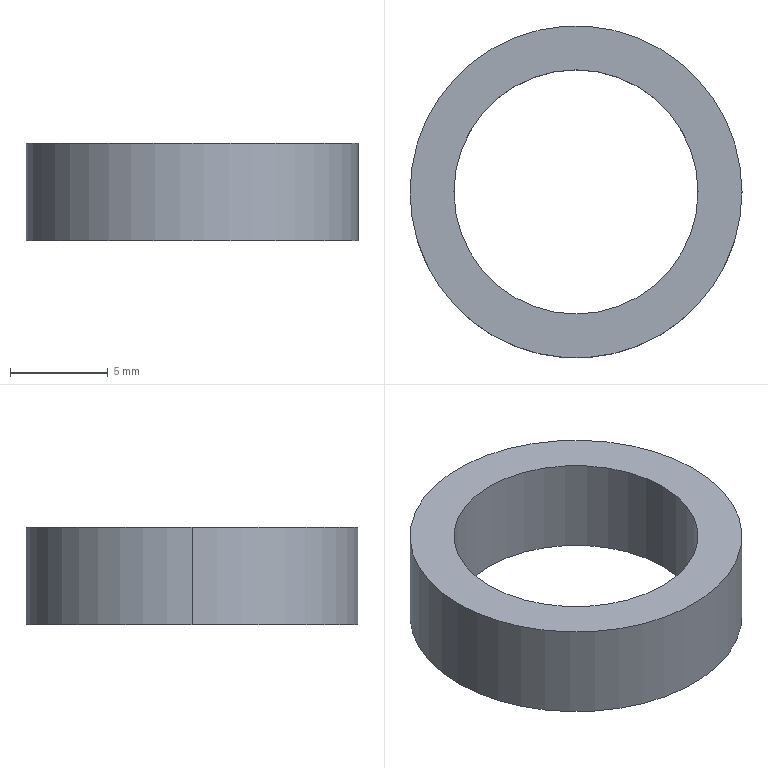Part | SolidWorks | features Extrusion 1 | 1 solid | 6 faces | box 17 x 17 x 5 mm | volume 521.308 mm3 | cylinder 4 | plane 2 | commonest cylinder face diameters 12.5 x2 17 x2
STEP:
#1=CARTESIAN_POINT('',(-6.25,0.,5.));
#2=VERTEX_POINT('',#1);
#3=CARTESIAN_POINT('',(6.25,0.,5.));
#4=VERTEX_POINT('',#3);
#5=CARTESIAN_POINT('',(0.,0.,5.));
#6=DIRECTION('',(0.,0.,1.));
#7=DIRECTION('',(1.,0.,0.));
#8=AXIS2_PLACEMENT_3D('',#5,#6,#7);
#9=CIRCLE('',#8,6.25);
#10=EDGE_CURVE('',#2,#4,#9,.T.);
#11=ORIENTED_EDGE('',*,*,#10,.T.);
#12=CARTESIAN_POINT('',(6.25,0.,0.));
#13=VERTEX_POINT('',#12);
#14=CARTESIAN_POINT('',(6.25,0.,5.));
#15=DIRECTION('',(0.,0.,-1.));
#16=VECTOR('',#15,1000.);
#17=LINE('',#14,#16);
#18=EDGE_CURVE('',#4,#13,#17,.T.);
#19=ORIENTED_EDGE('',*,*,#18,.T.);
#20=CARTESIAN_POINT('',(-6.25,0.,0.));
#21=VERTEX_POINT('',#20);
#22=CARTESIAN_POINT('',(0.,0.,0.));
#23=DIRECTION('',(0.,0.,1.));
#24=DIRECTION('',(1.,0.,0.));
#25=AXIS2_PLACEMENT_3D('',#22,#23,#24);
#26=CIRCLE('',#25,6.25);
#27=EDGE_CURVE('',#21,#13,#26,.T.);
#28=ORIENTED_EDGE('',*,*,#27,.F.);
#29=CARTESIAN_POINT('',(-6.25,0.,5.));
#30=DIRECTION('',(0.,0.,-1.));
#31=VECTOR('',#30,1000.);
#32=LINE('',#29,#31);
#33=EDGE_CURVE('',#2,#21,#32,.T.);
#34=ORIENTED_EDGE('',*,*,#33,.F.);
#35=EDGE_LOOP('',(#11,#19,#28,#34));
#36=FACE_OUTER_BOUND('',#35,.T.);
#37=CARTESIAN_POINT('',(0.,0.,5.));
#38=DIRECTION('',(0.,0.,-1.));
#39=DIRECTION('',(-1.,0.,0.));
#40=AXIS2_PLACEMENT_3D('',#37,#38,#39);
#41=CYLINDRICAL_SURFACE('',#40,6.25);
#42=ADVANCED_FACE('',(#36),#41,.F.);
#43=CARTESIAN_POINT('',(8.5,0.,5.));
#44=VERTEX_POINT('',#43);
#45=CARTESIAN_POINT('',(-8.5,0.,5.));
#46=VERTEX_POINT('',#45);
#47=CARTESIAN_POINT('',(0.,0.,5.));
#48=DIRECTION('',(0.,0.,1.));
#49=DIRECTION('',(1.,0.,0.));
#50=AXIS2_PLACEMENT_3D('',#47,#48,#49);
#51=CIRCLE('',#50,8.5);
#52=EDGE_CURVE('',#44,#46,#51,.T.);
#53=ORIENTED_EDGE('',*,*,#52,.F.);
#54=CARTESIAN_POINT('',(8.5,0.,0.));
#55=VERTEX_POINT('',#54);
#56=CARTESIAN_POINT('',(8.5,0.,5.));
#57=DIRECTION('',(0.,0.,-1.));
#58=VECTOR('',#57,1000.);
#59=LINE('',#56,#58);
#60=EDGE_CURVE('',#44,#55,#59,.T.);
#61=ORIENTED_EDGE('',*,*,#60,.T.);
#62=CARTESIAN_POINT('',(-8.5,0.,0.));
#63=VERTEX_POINT('',#62);
#64=CARTESIAN_POINT('',(0.,0.,0.));
#65=DIRECTION('',(0.,0.,1.));
#66=DIRECTION('',(1.,0.,0.));
#67=AXIS2_PLACEMENT_3D('',#64,#65,#66);
#68=CIRCLE('',#67,8.5);
#69=EDGE_CURVE('',#55,#63,#68,.T.);
#70=ORIENTED_EDGE('',*,*,#69,.T.);
#71=CARTESIAN_POINT('',(-8.5,0.,5.));
#72=DIRECTION('',(0.,0.,-1.));
#73=VECTOR('',#72,1000.);
#74=LINE('',#71,#73);
#75=EDGE_CURVE('',#46,#63,#74,.T.);
#76=ORIENTED_EDGE('',*,*,#75,.F.);
#77=EDGE_LOOP('',(#53,#61,#70,#76));
#78=FACE_OUTER_BOUND('',#77,.T.);
#79=CARTESIAN_POINT('',(0.,0.,5.));
#80=DIRECTION('',(0.,0.,-1.));
#81=DIRECTION('',(-1.,0.,0.));
#82=AXIS2_PLACEMENT_3D('',#79,#80,#81);
#83=CYLINDRICAL_SURFACE('',#82,8.5);
#84=ADVANCED_FACE('',(#78),#83,.T.);
#85=CARTESIAN_POINT('',(0.,0.,5.));
#86=DIRECTION('',(0.,0.,1.));
#87=DIRECTION('',(1.,0.,0.));
#88=AXIS2_PLACEMENT_3D('',#85,#86,#87);
#89=CIRCLE('',#88,8.5);
#90=EDGE_CURVE('',#46,#44,#89,.T.);
#91=ORIENTED_EDGE('',*,*,#90,.T.);
#92=ORIENTED_EDGE('',*,*,#52,.T.);
#93=EDGE_LOOP('',(#91,#92));
#94=FACE_OUTER_BOUND('',#93,.T.);
#95=ORIENTED_EDGE('',*,*,#10,.F.);
#96=CARTESIAN_POINT('',(0.,0.,5.));
#97=DIRECTION('',(0.,0.,1.));
#98=DIRECTION('',(1.,0.,0.));
#99=AXIS2_PLACEMENT_3D('',#96,#97,#98);
#100=CIRCLE('',#99,6.25);
#101=EDGE_CURVE('',#4,#2,#100,.T.);
#102=ORIENTED_EDGE('',*,*,#101,.F.);
#103=EDGE_LOOP('',(#95,#102));
#104=FACE_BOUND('',#103,.T.);
#105=CARTESIAN_POINT('',(0.,0.,5.));
#106=DIRECTION('',(0.,0.,1.));
#107=DIRECTION('',(1.,0.,0.));
#108=AXIS2_PLACEMENT_3D('',#105,#106,#107);
#109=PLANE('',#108);
#110=ADVANCED_FACE('',(#94,#104),#109,.T.);
#111=CARTESIAN_POINT('',(0.,0.,0.));
#112=DIRECTION('',(0.,0.,1.));
#113=DIRECTION('',(1.,0.,0.));
#114=AXIS2_PLACEMENT_3D('',#111,#112,#113);
#115=CIRCLE('',#114,8.5);
#116=EDGE_CURVE('',#63,#55,#115,.T.);
#117=ORIENTED_EDGE('',*,*,#116,.F.);
#118=ORIENTED_EDGE('',*,*,#69,.F.);
#119=EDGE_LOOP('',(#117,#118));
#120=FACE_OUTER_BOUND('',#119,.T.);
#121=ORIENTED_EDGE('',*,*,#27,.T.);
#122=CARTESIAN_POINT('',(0.,0.,0.));
#123=DIRECTION('',(0.,0.,1.));
#124=DIRECTION('',(1.,0.,0.));
#125=AXIS2_PLACEMENT_3D('',#122,#123,#124);
#126=CIRCLE('',#125,6.25);
#127=EDGE_CURVE('',#13,#21,#126,.T.);
#128=ORIENTED_EDGE('',*,*,#127,.T.);
#129=EDGE_LOOP('',(#121,#128));
#130=FACE_BOUND('',#129,.T.);
#131=CARTESIAN_POINT('',(0.,0.,0.));
#132=DIRECTION('',(0.,0.,1.));
#133=DIRECTION('',(1.,0.,0.));
#134=AXIS2_PLACEMENT_3D('',#131,#132,#133);
#135=PLANE('',#134);
#136=ADVANCED_FACE('',(#120,#130),#135,.F.);
#137=ORIENTED_EDGE('',*,*,#60,.F.);
#138=ORIENTED_EDGE('',*,*,#90,.F.);
#139=ORIENTED_EDGE('',*,*,#75,.T.);
#140=ORIENTED_EDGE('',*,*,#116,.T.);
#141=EDGE_LOOP('',(#137,#138,#139,#140));
#142=FACE_OUTER_BOUND('',#141,.T.);
#143=CARTESIAN_POINT('',(0.,0.,5.));
#144=DIRECTION('',(0.,0.,-1.));
#145=DIRECTION('',(-1.,0.,0.));
#146=AXIS2_PLACEMENT_3D('',#143,#144,#145);
#147=CYLINDRICAL_SURFACE('',#146,8.5);
#148=ADVANCED_FACE('',(#142),#147,.T.);
#149=ORIENTED_EDGE('',*,*,#18,.F.);
#150=ORIENTED_EDGE('',*,*,#101,.T.);
#151=ORIENTED_EDGE('',*,*,#33,.T.);
#152=ORIENTED_EDGE('',*,*,#127,.F.);
#153=EDGE_LOOP('',(#149,#150,#151,#152));
#154=FACE_OUTER_BOUND('',#153,.T.);
#155=CARTESIAN_POINT('',(0.,0.,5.));
#156=DIRECTION('',(0.,0.,-1.));
#157=DIRECTION('',(-1.,0.,0.));
#158=AXIS2_PLACEMENT_3D('',#155,#156,#157);
#159=CYLINDRICAL_SURFACE('',#158,6.25);
#160=ADVANCED_FACE('',(#154),#159,.F.);
#161=CLOSED_SHELL('',(#42,#84,#110,#136,#148,#160));
#162=MANIFOLD_SOLID_BREP('',#161);
#163=CARTESIAN_POINT('',(0.,0.,0.));
#164=DIRECTION('',(0.,0.,1.));
#165=DIRECTION('',(1.,0.,0.));
#166=AXIS2_PLACEMENT_3D('',#163,#164,#165);
#167=(LENGTH_UNIT()NAMED_UNIT(*)SI_UNIT(.MILLI.,.METRE.));
#168=UNCERTAINTY_MEASURE_WITH_UNIT(LENGTH_MEASURE(0.00001),#167,'','');
#169=(NAMED_UNIT(*)PLANE_ANGLE_UNIT()SI_UNIT($,.RADIAN.));
#170=(NAMED_UNIT(*)SI_UNIT($,.STERADIAN.)SOLID_ANGLE_UNIT());
#171=(GEOMETRIC_REPRESENTATION_CONTEXT(3)GLOBAL_UNCERTAINTY_ASSIGNED_CONTEXT((#168))GLOBAL_UNIT_ASSIGNED_CONTEXT((#167,#169,#170))REPRESENTATION_CONTEXT('',''));
#172=ADVANCED_BREP_SHAPE_REPRESENTATION('',(#162,#166),#171);